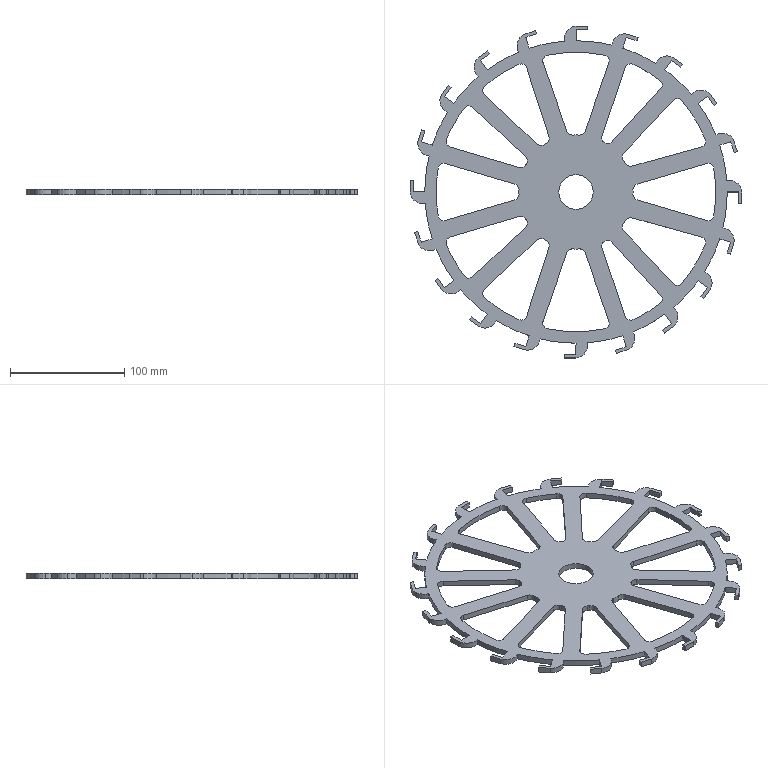Part | SolidWorks | features ICE 2, Extrusion 1, Fillet 1 | 1 solid | 239 faces | box 291 x 291 x 5 mm | volume 156823 mm3 | cylinder 133 | plane 106 | commonest cylinder face diameters 10 x60 22 x25 265 x20 100 x13 245 x13 30.2 x2